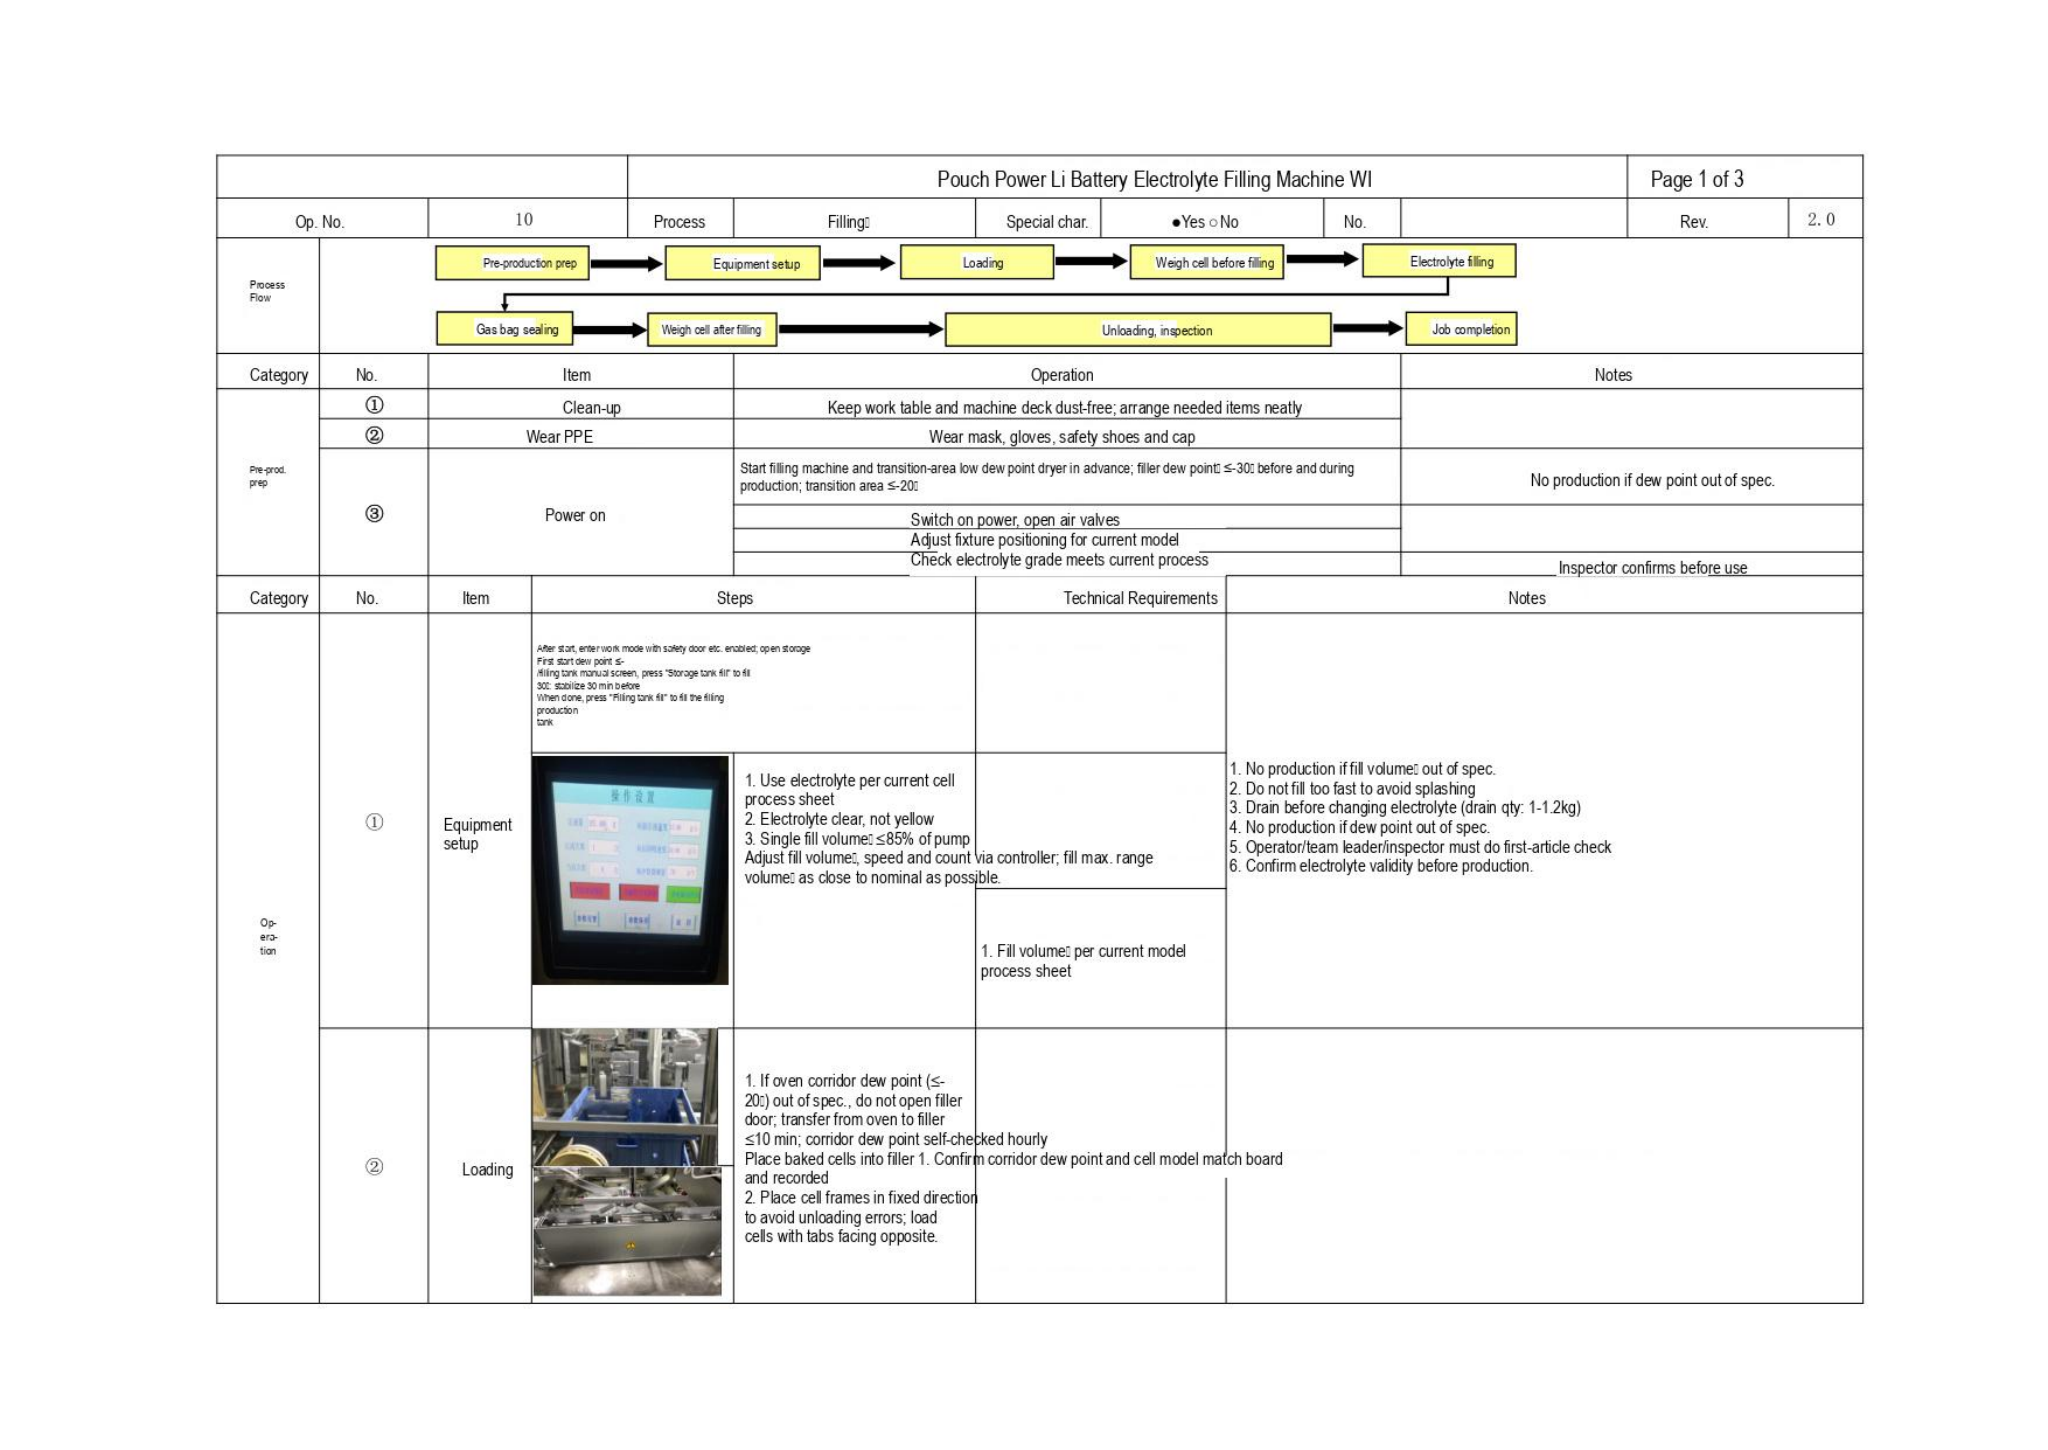| | Pouch Power Li Battery Electrolyte Filling Machine WI | | | | | | | Page 1 of 3 | |
|---|---|---|---|---|---|---|---|---|---|
| Op. No. | 10 | Process | Filling | Special char. | ●Yes ○No | No. | | Rev. | 2.0 |

Process Flow

Pre-production prep → Equipment setup → Loading → Weigh cell before filling → Electrolyte filling → Gas bag sealing → Weigh cell after filling → Unloading, inspection → Job completion

| Category | No. | Item | Operation | Notes |
|---|---|---|---|---|
| Pre-prod. prep | ① | Clean-up | Keep work table and machine deck dust-free; arrange needed items neatly | |
| | ② | Wear PPE | Wear mask, gloves, safety shoes and cap | |
| | ③ | Power on | Start filling machine and transition-area low dew point dryer in advance; filler dew point ≤-30 before and during production; transition area ≤-20 | No production if dew point out of spec. |
| | | | Switch on power, open air valves | |
| | | | Adjust fixture positioning for current model | |
| | | | Check electrolyte grade meets current process | Inspector confirms before use |

| Category | No. | Item | Steps | Technical Requirements | Notes |
|---|---|---|---|---|---|
| Operation | ① | Equipment setup | After start, enter work mode with safety door etc. enabled; open storage<br>First start dew point ≤-<br>filling tank manual screen, press "Storage tank fill" to fill<br>30: stabilize 30 min before<br>When done, press "Filling tank fill" to fill the filling<br>production<br>tank | | 1. No production if fill volume out of spec.<br>2. Do not fill too fast to avoid splashing<br>3. Drain before changing electrolyte (drain qty: 1-1.2kg)<br>4. No production if dew point out of spec.<br>5. Operator/team leader/inspector must do first-article check<br>6. Confirm electrolyte validity before production. |
| | | | 1. Use electrolyte per current cell process sheet<br>2. Electrolyte clear, not yellow<br>3. Single fill volume ≤85% of pump<br>Adjust fill volume, speed and count via controller; fill max. range volume as close to nominal as possible. | 1. Fill volume per current model process sheet | |
| | ② | Loading | 1. If oven corridor dew point (≤-20) out of spec., do not open filler door; transfer from oven to filler ≤10 min; corridor dew point self-checked hourly<br>Place baked cells into filler<br>2. Place cell frames in fixed direction to avoid unloading errors; load cells with tabs facing opposite. | 1. Confirm corridor dew point and cell model match board and recorded | |
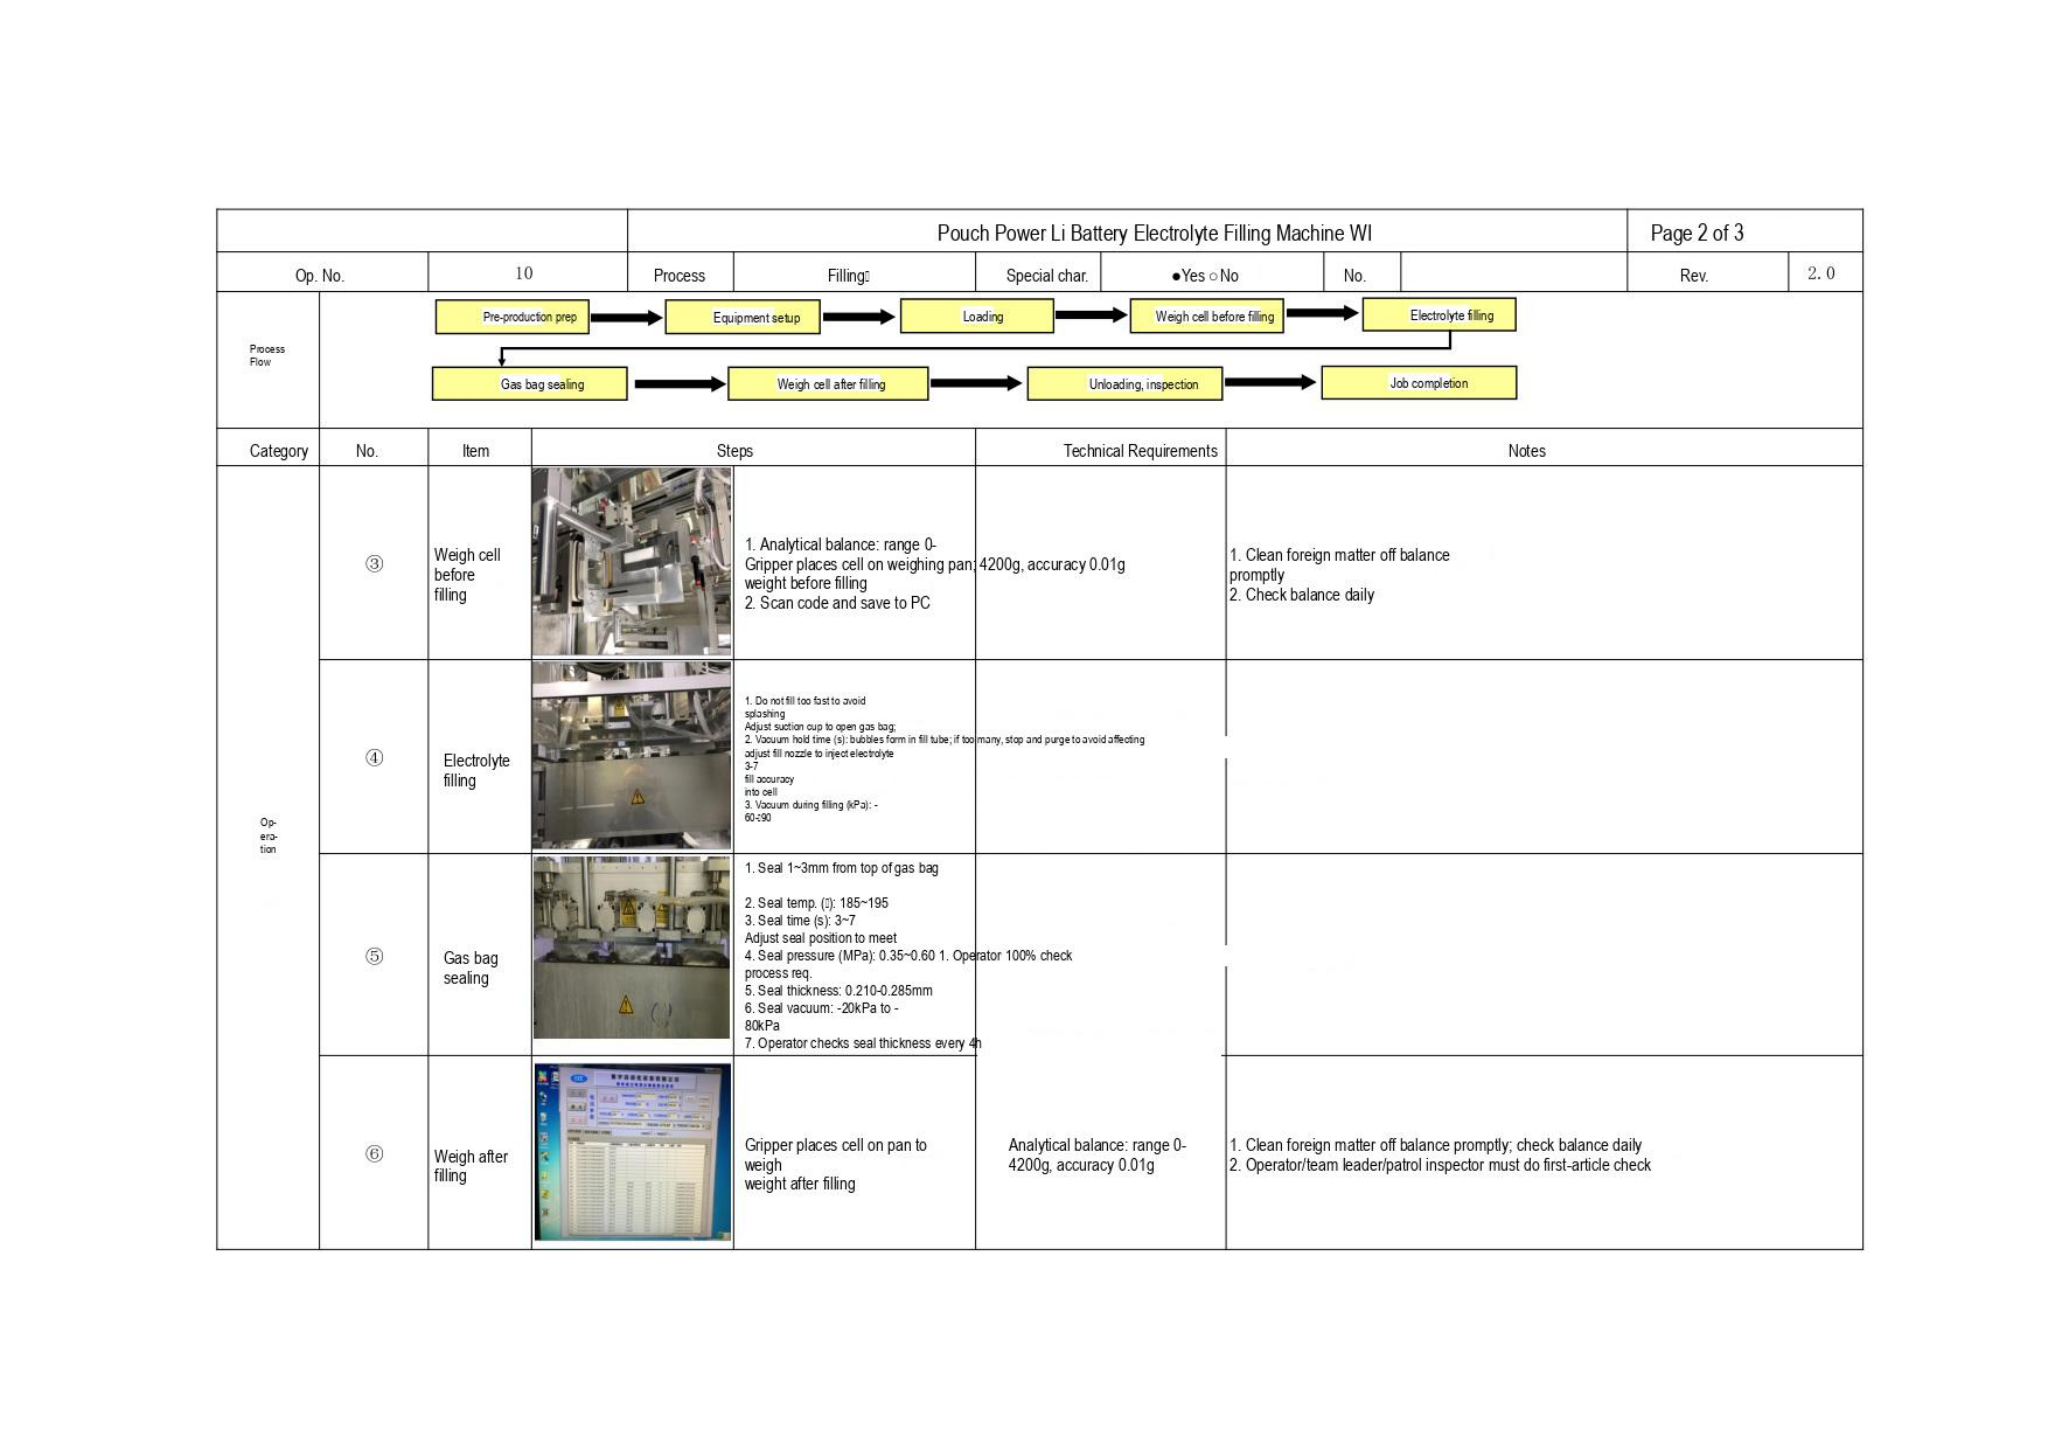| | | | | | | | | | |
|---|---|---|---|---|---|---|---|---|---|
| | | Pouch Power Li Battery Electrolyte Filling Machine WI | | | | | | Page 2 of 3 | |
| Op. No. | 10 | Process | Filling | Special char. | ●Yes ○No | No. | | Rev. | 2.0 |

Process Flow

Pre-production prep → Equipment setup → Loading → Weigh cell before filling → Electrolyte filling → Gas bag sealing → Weigh cell after filling → Unloading, inspection → Job completion

| Category | No. | Item | Steps | Technical Requirements | Notes |
|---|---|---|---|---|---|
| Op-<br>era-<br>tion | ③ | Weigh cell before filling | 1. Analytical balance: range 0-<br>Gripper places cell on weighing pan;<br>weight before filling<br>2. Scan code and save to PC | 4200g, accuracy 0.01g | 1. Clean foreign matter off balance promptly<br>2. Check balance daily |
| | ④ | Electrolyte filling | 1. Do not fill too fast to avoid splashing<br>Adjust suction cup to open gas bag;<br>2. Vacuum hold time (s): bubbles form in fill tube; if too many, stop and purge to avoid affecting<br>adjust fill nozzle to inject electrolyte<br>3-7<br>fill accuracy<br>into cell<br>3. Vacuum during filling (kPa): -<br>60-90 | | |
| | ⑤ | Gas bag sealing | 1. Seal 1~3mm from top of gas bag<br>2. Seal temp. (): 185~195<br>3. Seal time (s): 3~7<br>Adjust seal position to meet<br>4. Seal pressure (MPa): 0.35~0.60 1. Operator 100% check<br>process req.<br>5. Seal thickness: 0.210-0.285mm<br>6. Seal vacuum: -20kPa to -<br>80kPa<br>7. Operator checks seal thickness every 4h | | |
| | ⑥ | Weigh after filling | Gripper places cell on pan to weigh<br>weight after filling | Analytical balance: range 0-4200g, accuracy 0.01g | 1. Clean foreign matter off balance promptly; check balance daily<br>2. Operator/team leader/patrol inspector must do first-article check |
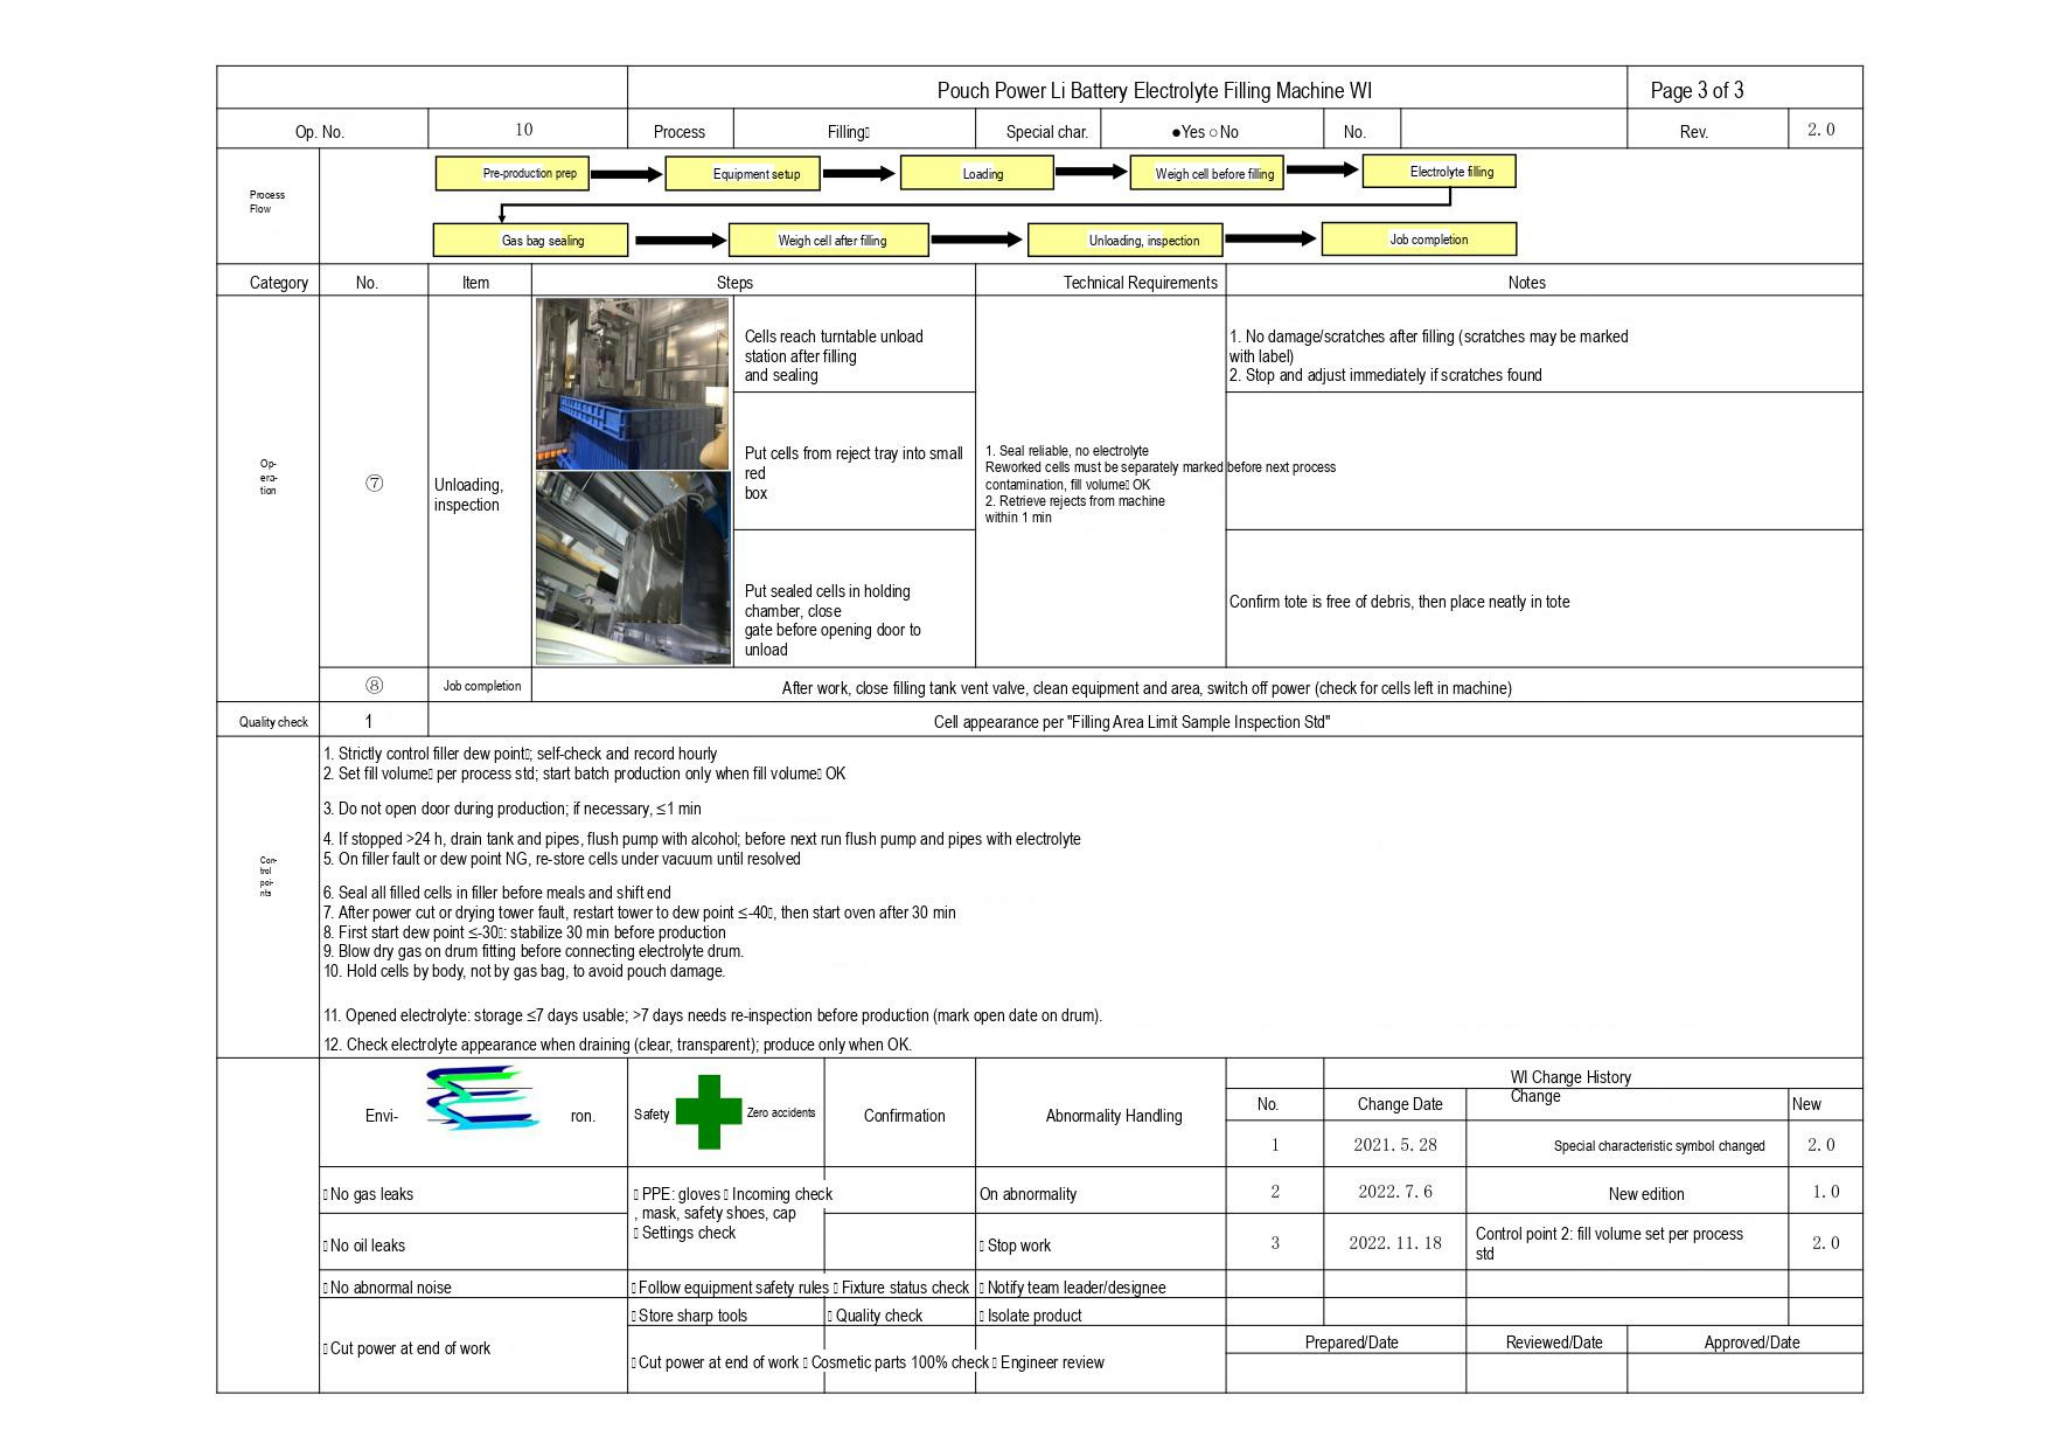Pouch Power Li Battery Electrolyte Filling Machine WI

Page 3 of 3

| Op. No. | 10 | Process | Filling | Special char. | ●Yes ○No | No. | | Rev. | 2. 0 |
|---|---|---|---|---|---|---|---|---|---|

Process Flow

Pre-production prep → Equipment setup → Loading → Weigh cell before filling → Electrolyte filling → Gas bag sealing → Weigh cell after filling → Unloading, inspection → Job completion

| Category | No. | Item | Steps | Technical Requirements | Notes |
|---|---|---|---|---|---|
| Op-era-tion | ⑦ | Unloading, inspection | Cells reach turntable unload station after filling and sealing | 1. Seal reliable, no electrolyte contamination, fill volume OK<br>2. Retrieve rejects from machine within 1 min | 1. No damage/scratches after filling (scratches may be marked with label)<br>2. Stop and adjust immediately if scratches found |
| | | | Put cells from reject tray into small red box | | Reworked cells must be separately marked before next process |
| | | | Put sealed cells in holding chamber, close gate before opening door to unload | | Confirm tote is free of debris, then place neatly in tote |
| | ⑧ | Job completion | After work, close filling tank vent valve, clean equipment and area, switch off power (check for cells left in machine) | | |
| Quality check | 1 | Cell appearance per "Filling Area Limit Sample Inspection Std" | | | |

Con-trol poi-nts

1. Strictly control filler dew point; self-check and record hourly
2. Set fill volume per process std; start batch production only when fill volume OK
3. Do not open door during production; if necessary, ≤1 min
4. If stopped >24 h, drain tank and pipes, flush pump with alcohol; before next run flush pump and pipes with electrolyte
5. On filler fault or dew point NG, re-store cells under vacuum until resolved
6. Seal all filled cells in filler before meals and shift end
7. After power cut or drying tower fault, restart tower to dew point ≤-40, then start oven after 30 min
8. First start dew point ≤-30: stabilize 30 min before production
9. Blow dry gas on drum fitting before connecting electrolyte drum.
10. Hold cells by body, not by gas bag, to avoid pouch damage.
11. Opened electrolyte: storage ≤7 days usable; >7 days needs re-inspection before production (mark open date on drum).
12. Check electrolyte appearance when draining (clear, transparent); produce only when OK.

| Envi- ron. | Safety Zero accidents | Confirmation | Abnormality Handling |
|---|---|---|---|
| No gas leaks | PPE: gloves, mask, safety shoes, cap | Incoming check | On abnormality |
| No oil leaks | Settings check | | Stop work |
| No abnormal noise | Follow equipment safety rules | Fixture status check | Notify team leader/designee |
| | Store sharp tools | Quality check | Isolate product |
| Cut power at end of work | Cut power at end of work | Cosmetic parts 100% check | Engineer review |

WI Change History

| No. | Change Date | Change | New |
|---|---|---|---|
| 1 | 2021. 5. 28 | Special characteristic symbol changed | 2. 0 |
| 2 | 2022. 7. 6 | New edition | 1. 0 |
| 3 | 2022. 11. 18 | Control point 2: fill volume set per process std | 2. 0 |

| Prepared/Date | Reviewed/Date | Approved/Date |
|---|---|---|
| | | |